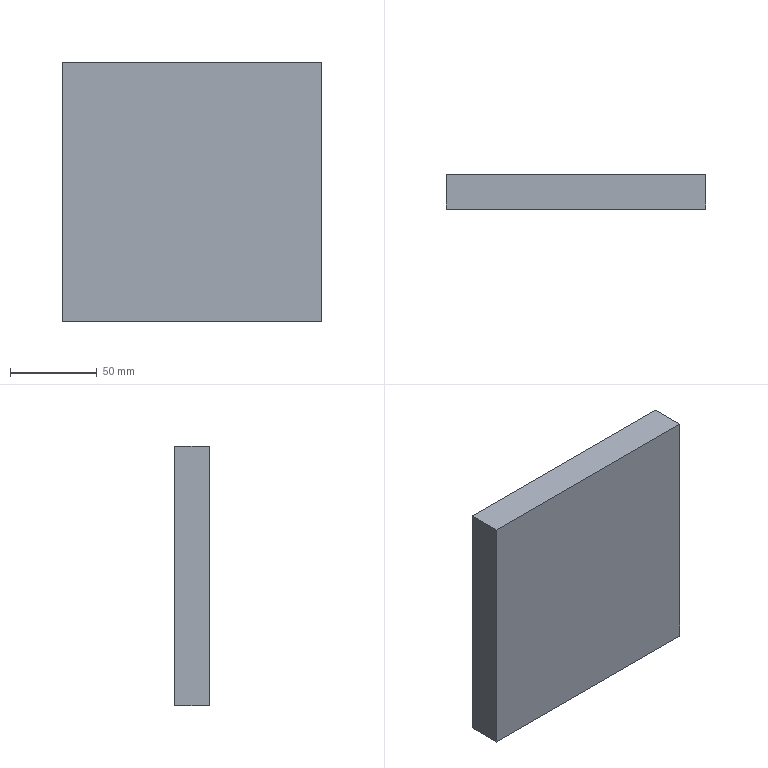Part | NX | features solid 2 | 1 solid | 6 faces | box 150 x 20 x 150 mm | volume 450000 mm3 | plane 6
STEP:
#1=CARTESIAN_POINT('',(-1385.,-530.,-310.));
#2=VERTEX_POINT('',#1);
#3=CARTESIAN_POINT('',(-1535.,-530.,-310.));
#4=VERTEX_POINT('',#3);
#5=CARTESIAN_POINT('',(-1410.,-530.,-310.));
#6=DIRECTION('',(-1.,0.,0.));
#7=VECTOR('',#6,1000.);
#8=LINE('',#5,#7);
#9=EDGE_CURVE('',#2,#4,#8,.T.);
#10=ORIENTED_EDGE('',*,*,#9,.F.);
#11=CARTESIAN_POINT('',(-1385.,-550.,-310.));
#12=VERTEX_POINT('',#11);
#13=CARTESIAN_POINT('',(-1385.,-550.,-310.));
#14=DIRECTION('',(0.,1.,0.));
#15=VECTOR('',#14,1000.);
#16=LINE('',#13,#15);
#17=EDGE_CURVE('',#12,#2,#16,.T.);
#18=ORIENTED_EDGE('',*,*,#17,.F.);
#19=CARTESIAN_POINT('',(-1535.,-550.,-310.));
#20=VERTEX_POINT('',#19);
#21=CARTESIAN_POINT('',(-1410.,-550.,-310.));
#22=DIRECTION('',(-1.,0.,0.));
#23=VECTOR('',#22,1000.);
#24=LINE('',#21,#23);
#25=EDGE_CURVE('',#12,#20,#24,.T.);
#26=ORIENTED_EDGE('',*,*,#25,.T.);
#27=CARTESIAN_POINT('',(-1535.,-550.,-310.));
#28=DIRECTION('',(0.,1.,0.));
#29=VECTOR('',#28,1000.);
#30=LINE('',#27,#29);
#31=EDGE_CURVE('',#20,#4,#30,.T.);
#32=ORIENTED_EDGE('',*,*,#31,.T.);
#33=EDGE_LOOP('',(#10,#18,#26,#32));
#34=FACE_BOUND('',#33,.T.);
#35=CARTESIAN_POINT('',(-1410.,-550.,-310.));
#36=DIRECTION('',(0.,0.,1.));
#37=DIRECTION('',(1.,0.,0.));
#38=AXIS2_PLACEMENT_3D('',#35,#36,#37);
#39=PLANE('',#38);
#40=ADVANCED_FACE('',(#34),#39,.F.);
#41=CARTESIAN_POINT('',(-1535.,-530.,-160.));
#42=VERTEX_POINT('',#41);
#43=CARTESIAN_POINT('',(-1535.,-530.,-200.));
#44=DIRECTION('',(0.,0.,1.));
#45=VECTOR('',#44,1000.);
#46=LINE('',#43,#45);
#47=EDGE_CURVE('',#4,#42,#46,.T.);
#48=ORIENTED_EDGE('',*,*,#47,.F.);
#49=ORIENTED_EDGE('',*,*,#31,.F.);
#50=CARTESIAN_POINT('',(-1535.,-550.,-160.));
#51=VERTEX_POINT('',#50);
#52=CARTESIAN_POINT('',(-1535.,-550.,-200.));
#53=DIRECTION('',(0.,0.,1.));
#54=VECTOR('',#53,1000.);
#55=LINE('',#52,#54);
#56=EDGE_CURVE('',#20,#51,#55,.T.);
#57=ORIENTED_EDGE('',*,*,#56,.T.);
#58=CARTESIAN_POINT('',(-1535.,-550.,-160.));
#59=DIRECTION('',(0.,1.,0.));
#60=VECTOR('',#59,1000.);
#61=LINE('',#58,#60);
#62=EDGE_CURVE('',#51,#42,#61,.T.);
#63=ORIENTED_EDGE('',*,*,#62,.T.);
#64=EDGE_LOOP('',(#48,#49,#57,#63));
#65=FACE_BOUND('',#64,.T.);
#66=CARTESIAN_POINT('',(-1535.,-550.,-200.));
#67=DIRECTION('',(1.,0.,0.));
#68=DIRECTION('',(0.,0.,-1.));
#69=AXIS2_PLACEMENT_3D('',#66,#67,#68);
#70=PLANE('',#69);
#71=ADVANCED_FACE('',(#65),#70,.F.);
#72=CARTESIAN_POINT('',(-1385.,-530.,-160.));
#73=VERTEX_POINT('',#72);
#74=CARTESIAN_POINT('',(-1510.,-530.,-160.));
#75=DIRECTION('',(1.,0.,0.));
#76=VECTOR('',#75,1000.);
#77=LINE('',#74,#76);
#78=EDGE_CURVE('',#42,#73,#77,.T.);
#79=ORIENTED_EDGE('',*,*,#78,.F.);
#80=ORIENTED_EDGE('',*,*,#62,.F.);
#81=CARTESIAN_POINT('',(-1385.,-550.,-160.));
#82=VERTEX_POINT('',#81);
#83=CARTESIAN_POINT('',(-1510.,-550.,-160.));
#84=DIRECTION('',(1.,0.,0.));
#85=VECTOR('',#84,1000.);
#86=LINE('',#83,#85);
#87=EDGE_CURVE('',#51,#82,#86,.T.);
#88=ORIENTED_EDGE('',*,*,#87,.T.);
#89=CARTESIAN_POINT('',(-1385.,-550.,-160.));
#90=DIRECTION('',(0.,1.,0.));
#91=VECTOR('',#90,1000.);
#92=LINE('',#89,#91);
#93=EDGE_CURVE('',#82,#73,#92,.T.);
#94=ORIENTED_EDGE('',*,*,#93,.T.);
#95=EDGE_LOOP('',(#79,#80,#88,#94));
#96=FACE_BOUND('',#95,.T.);
#97=CARTESIAN_POINT('',(-1510.,-550.,-160.));
#98=DIRECTION('',(0.,0.,-1.));
#99=DIRECTION('',(0.,-1.,0.));
#100=AXIS2_PLACEMENT_3D('',#97,#98,#99);
#101=PLANE('',#100);
#102=ADVANCED_FACE('',(#96),#101,.F.);
#103=CARTESIAN_POINT('',(-1385.,-530.,-200.));
#104=DIRECTION('',(0.,0.,-1.));
#105=VECTOR('',#104,1000.);
#106=LINE('',#103,#105);
#107=EDGE_CURVE('',#73,#2,#106,.T.);
#108=ORIENTED_EDGE('',*,*,#107,.F.);
#109=ORIENTED_EDGE('',*,*,#93,.F.);
#110=CARTESIAN_POINT('',(-1385.,-550.,-200.));
#111=DIRECTION('',(0.,0.,-1.));
#112=VECTOR('',#111,1000.);
#113=LINE('',#110,#112);
#114=EDGE_CURVE('',#82,#12,#113,.T.);
#115=ORIENTED_EDGE('',*,*,#114,.T.);
#116=ORIENTED_EDGE('',*,*,#17,.T.);
#117=EDGE_LOOP('',(#108,#109,#115,#116));
#118=FACE_BOUND('',#117,.T.);
#119=CARTESIAN_POINT('',(-1385.,-550.,-100.));
#120=DIRECTION('',(-1.,0.,0.));
#121=DIRECTION('',(0.,0.,1.));
#122=AXIS2_PLACEMENT_3D('',#119,#120,#121);
#123=PLANE('',#122);
#124=ADVANCED_FACE('',(#118),#123,.F.);
#125=ORIENTED_EDGE('',*,*,#25,.F.);
#126=ORIENTED_EDGE('',*,*,#114,.F.);
#127=ORIENTED_EDGE('',*,*,#87,.F.);
#128=ORIENTED_EDGE('',*,*,#56,.F.);
#129=EDGE_LOOP('',(#125,#126,#127,#128));
#130=FACE_BOUND('',#129,.T.);
#131=CARTESIAN_POINT('',(-1510.,-550.,-200.));
#132=DIRECTION('',(0.,-1.,0.));
#133=DIRECTION('',(1.,0.,0.));
#134=AXIS2_PLACEMENT_3D('',#131,#132,#133);
#135=PLANE('',#134);
#136=ADVANCED_FACE('',(#130),#135,.T.);
#137=ORIENTED_EDGE('',*,*,#9,.T.);
#138=ORIENTED_EDGE('',*,*,#47,.T.);
#139=ORIENTED_EDGE('',*,*,#78,.T.);
#140=ORIENTED_EDGE('',*,*,#107,.T.);
#141=EDGE_LOOP('',(#137,#138,#139,#140));
#142=FACE_BOUND('',#141,.T.);
#143=CARTESIAN_POINT('',(-1510.,-530.,-200.));
#144=DIRECTION('',(0.,-1.,0.));
#145=DIRECTION('',(1.,0.,0.));
#146=AXIS2_PLACEMENT_3D('',#143,#144,#145);
#147=PLANE('',#146);
#148=ADVANCED_FACE('',(#142),#147,.F.);
#149=CLOSED_SHELL('',(#40,#71,#102,#124,#136,#148));
#150=MANIFOLD_SOLID_BREP('',#149);
#151=(LENGTH_UNIT()NAMED_UNIT(*)SI_UNIT(.MILLI.,.METRE.));
#152=UNCERTAINTY_MEASURE_WITH_UNIT(LENGTH_MEASURE(0.00001),#151,'','');
#153=(NAMED_UNIT(*)PLANE_ANGLE_UNIT()SI_UNIT($,.RADIAN.));
#154=(NAMED_UNIT(*)SI_UNIT($,.STERADIAN.)SOLID_ANGLE_UNIT());
#155=(GEOMETRIC_REPRESENTATION_CONTEXT(3)GLOBAL_UNCERTAINTY_ASSIGNED_CONTEXT((#152))GLOBAL_UNIT_ASSIGNED_CONTEXT((#151,#153,#154))REPRESENTATION_CONTEXT('',''));
#156=ADVANCED_BREP_SHAPE_REPRESENTATION('',(#150),#155);